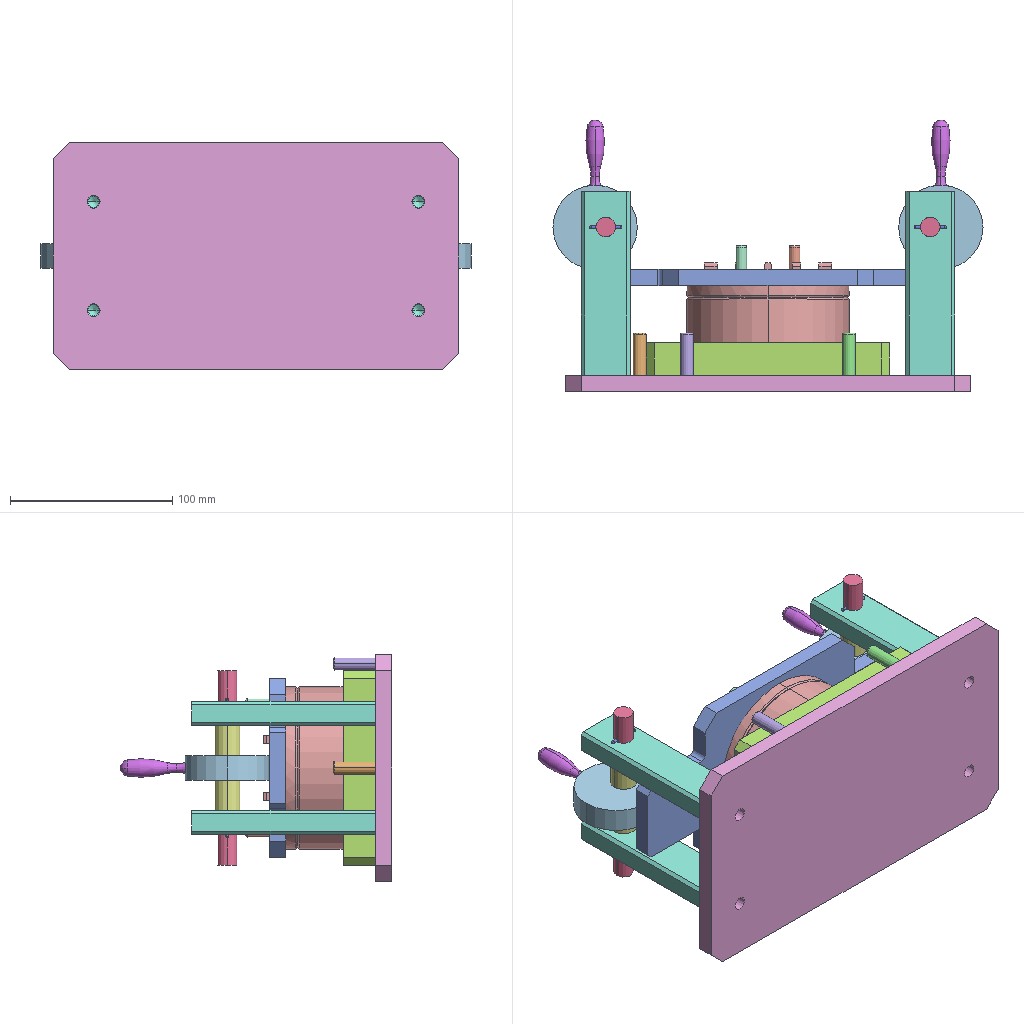Assembly | SolidWorks | 12 different items | 24 placed | box 265 x 167 x 140 mm
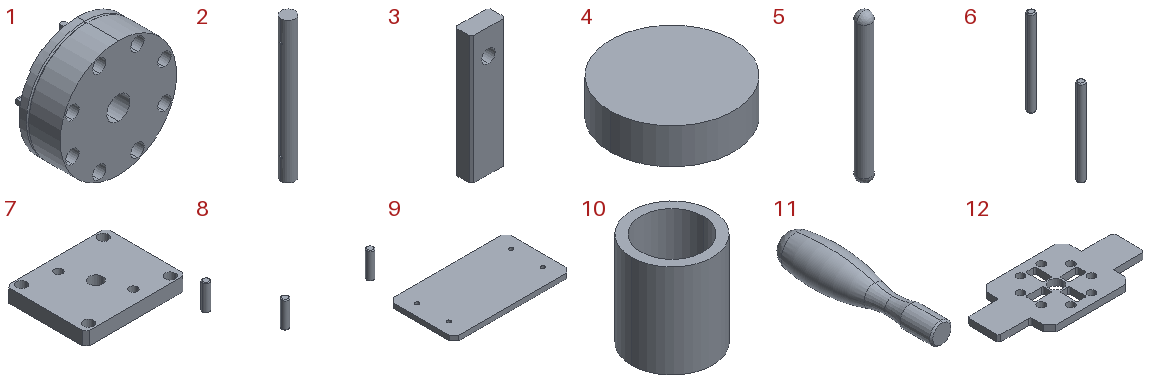Parts list (item | quantity | size | volume | features):
1 | x1 | 100 x 49.3 x 100 mm | 247149 mm3 | features ICE 7, CirPattern 4, RevCut 3, Chamfer 1, Extrusion 1, Fillet 1, MirrorPattern 1
2 | x2 | 12 x 12 x 120 mm | 13497 mm3 | features Cut 1, Extrusion 1
3 | x4 | 30 x 15 x 113.3 mm | 47736 mm3 | features Cut 1, Extrusion 1, HoleWzd 1
4 | x2 | 52 x 52 x 15 mm | 31469 mm3 | features Extrusion 1, RevCut 1
5 | x4 | 2 x 2 x 20 mm | 60.737 mm3 | features Extrusion 1, Fillet 1
6 | x1 | 39.358 x 85.684 x 80 mm | 5457 mm3 | features Fillet 2, Extrusion 1
7 | x1 | 150 x 120 x 20 mm | 334056 mm3 | features Cut 2, Extrusion 1, ICE 1
8 | x1 | 137.1 x 72.1 x 31 mm | 4644 mm3 | features Fillet 3, Extrusion 1
9 | x1 | 250 x 140 x 10 mm | 345235 mm3 | features Cut 2, ICE 2, Extrusion 1
10 | x4 | 16 x 16 x 18.5 mm | 1521 mm3 | features Extrusion 1
11 | x2 | 11.343 x 50 x 11.343 mm | 2889 mm3 | features Revolution 1
12 | x1 | 230 x 110 x 10 mm | 161829 mm3 | features Cut 1, Extrusion 1, Fillet 1, ICE 1
Mates (type | each side: item.copy, entity, surface, feature):
InPlace | 1.1 face plane Boss-Extrude1 | 12.1 plane
InPlace | 1.1 face plane Boss-Extrude1 | 7.1 plane
InPlace | 7.1 face plane Boss-Extrude1 | 9.1 plane
InPlace | 9.1 face plane Boss-Extrude1 | 3.1 plane
InPlace | 9.1 face plane Boss-Extrude1 | 8.1 plane
InPlace | 2.1 plane | assembly plane
InPlace | 4.1 plane | assembly plane
InPlace | 4.1 face plane Boss-Extrude1 | 10.1 plane
InPlace | 11.1 plane | assembly plane
InPlace | 9.1 face plane Boss-Extrude1 | 6.1 plane
InPlace | 3.2 face plane Boss-Extrude1 | 5.1 plane